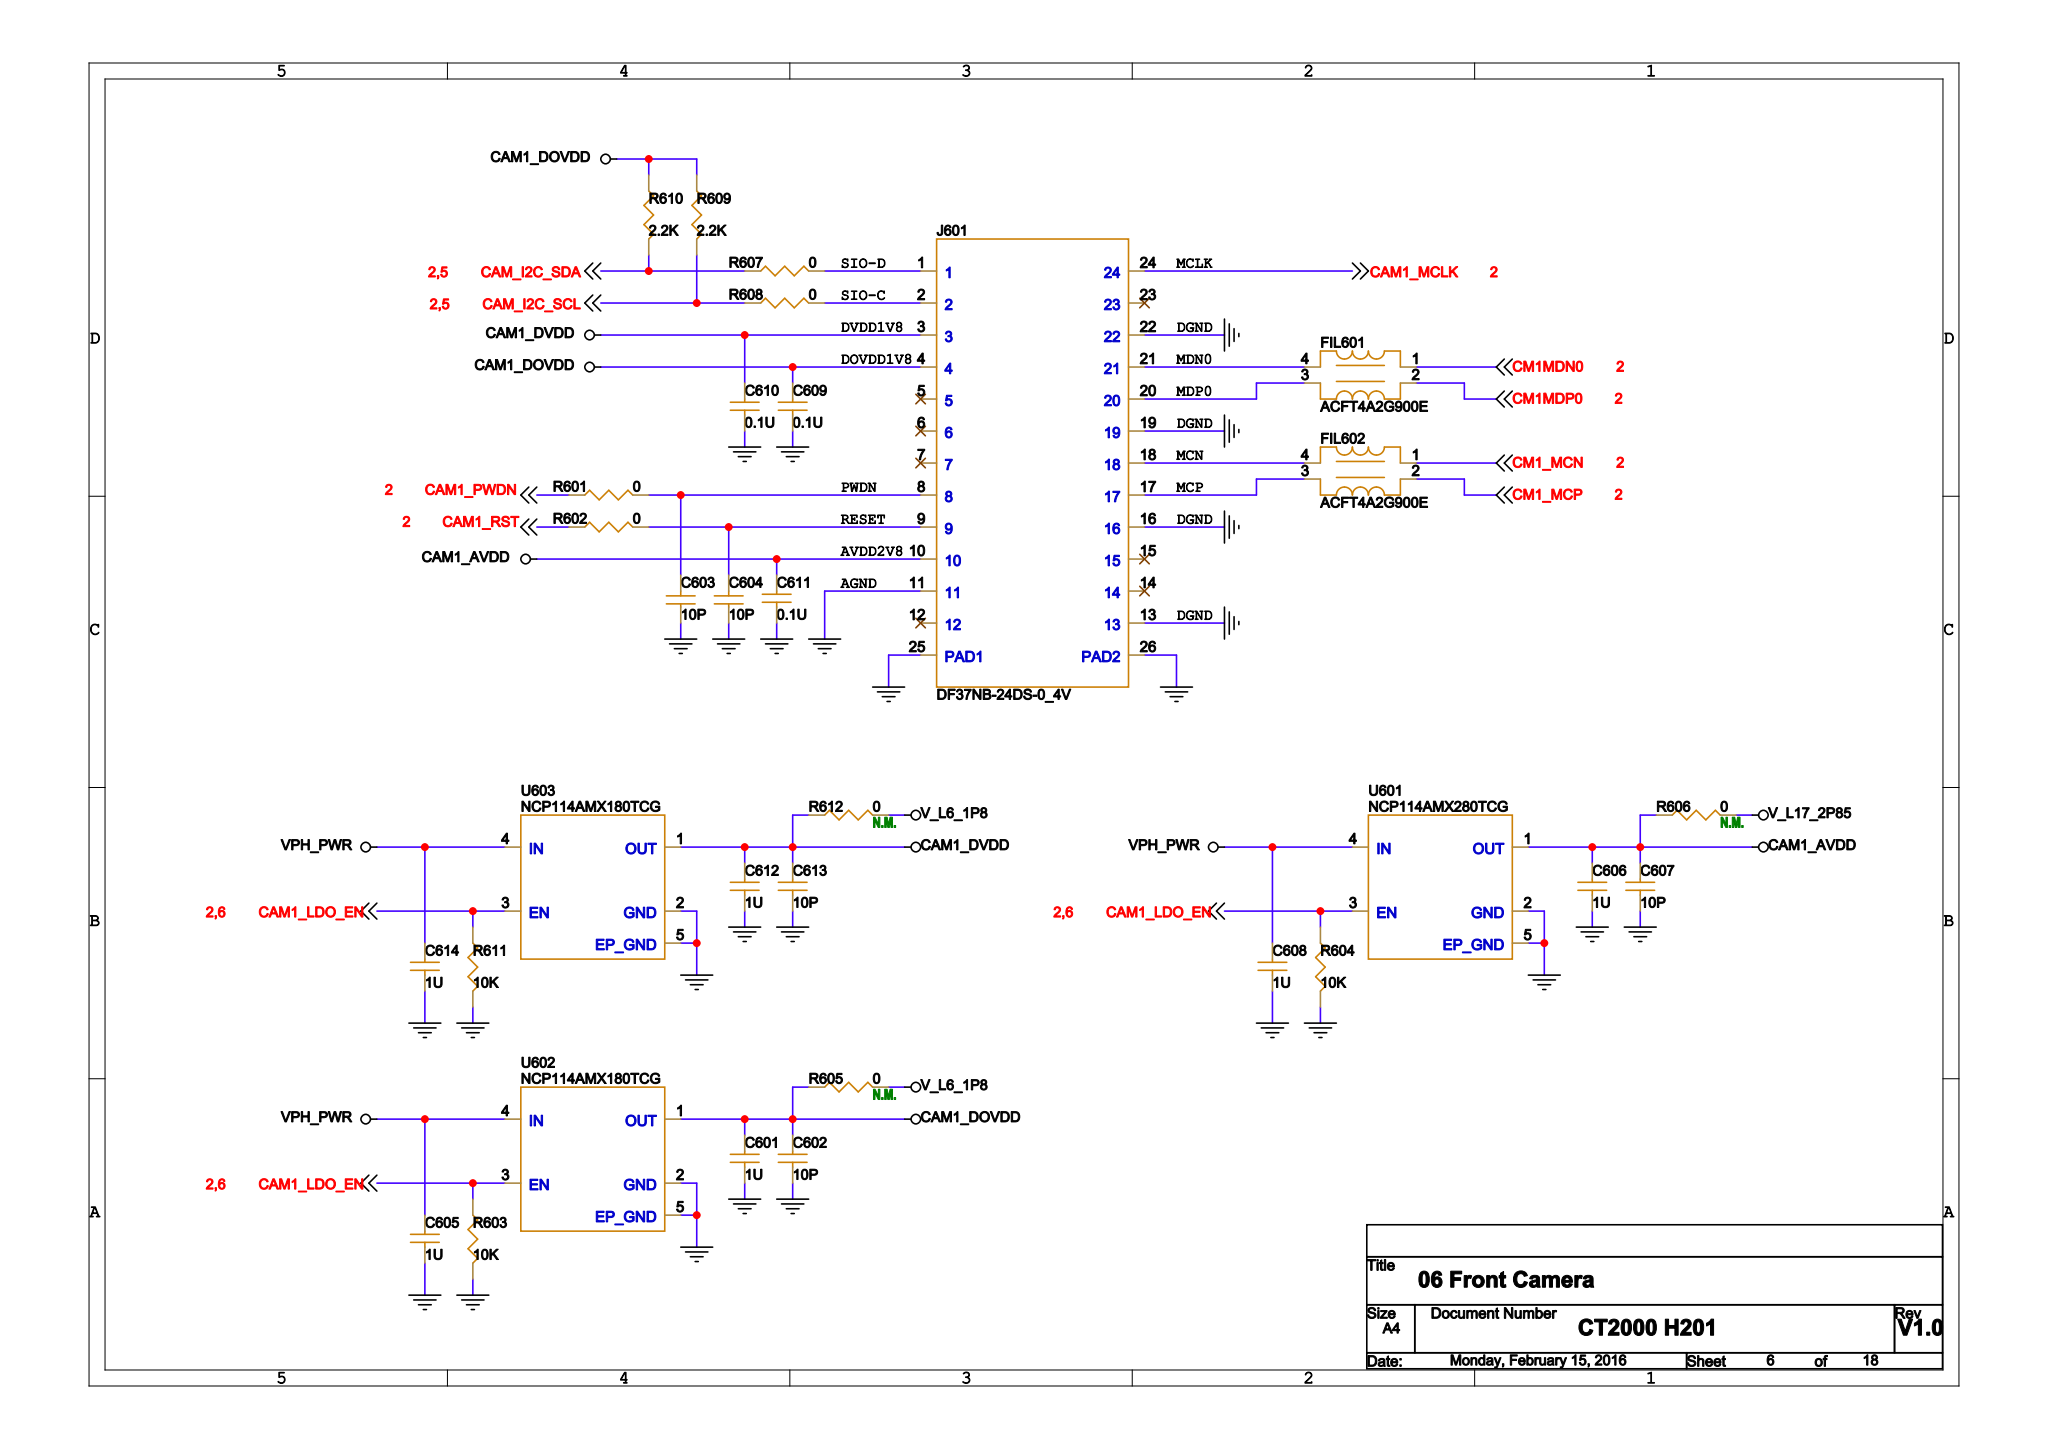Circuit board | Cadence Allegro | 573 parts | 376 nets | one sheet of the schematic
Parts on this sheet (reference | value | footprint):
C601 | 1U | C0402
C602 | 10P | C0402
C603 | 10P | C0402
C604 | 10P | C0402
C605 | 1U | C0402
C606 | 1U | C0402
C607 | 10P | C0402
C608 | 1U | C0402
C609 | 0.1U | C0402
C610 | 0.1U | C0402
C611 | 0.1U | C0402
C612 | 1U | C0402
C613 | 10P | C0402
C614 | 1U | C0402
FIL601 | ACFT4A2G900E | EMI4_0P85X0P65X0P55_INNOCHIPS
FIL602 | ACFT4A2G900E | EMI4_0P85X0P65X0P55_INNOCHIPS
J601 | DF37NB-24DS-0_4V | BTB_DF37NB-24DS-0_4V_CW
R601 | 0 | R0402
R602 | 0 | R0402
R603 | 10K | R0402
R604 | 10K | R0402
R605 | 0 | R0402
R606 | 0 | R0402
R607 | 0 | R0402
R608 | 0 | R0402
R609 | 2.2K | R0402
R610 | 2.2K | R0402
R611 | 10K | R0402
R612 | 0 | R0402
U601 | NCP114AMX280TCG | UDFN4_1X1X0P7_0P65
U602 | NCP114AMX180TCG | UDFN4_1X1X0P7_0P65
U603 | NCP114AMX180TCG | UDFN4_1X1X0P7_0P65
Nets of these parts (net: part-pin ...):
GND: C601-2 C602-2 C603-1 C604-1 C605-2 C606-2 C607-2 C608-2 C609-2 C610-2 C611-2 C612-2 C613-2 C614-2 J601-11 J601-13 J601-16 J601-19 J601-22 J601-25 J601-26 R603-2 R604-2 R611-2 U601-2 U601-5 U602-2 U602-5 U603-2 U603-5
V_L17_2P85: R606-1
VPH_PWR: C605-1 C608-1 C614-1 U601-4 U602-4 U603-4
CAM1_LDO_EN: R603-1 R604-1 R611-1 U601-3 U602-3 U603-3
CAM1_DOVDD: C601-1 C602-1 C609-1 J601-4 R605-2 R609-1 R610-1 U602-1
CAM1_DVDD: C610-1 C612-1 C613-1 J601-3 R612-2 U603-1
CAM1_PWDN: R601-1
CAM1_RST: R602-1
CAM_I2C_SDA: R607-1 R610-2
CAM_I2C_SCL: R608-1 R609-2
CM1_MCN: FIL602-1
CM1_MCP: FIL602-2
CM1MDN0: FIL601-1
CM1MDP0: FIL601-2
V_L6_1P8: R605-1 R612-1
N52162104: J601-1 R607-2
CAM1_AVDD: C606-1 C607-1 C611-1 J601-10 R606-2 U601-1
N52168904: FIL602-3 J601-17
N52168902: FIL602-4 J601-18
N52162106: J601-2 R608-2
N52161407: FIL601-3 J601-20
N52161405: FIL601-4 J601-21
CAM1_MCLK: J601-24
N52168249: C603-2 J601-8 R601-2
N52168120: C604-2 J601-9 R602-2